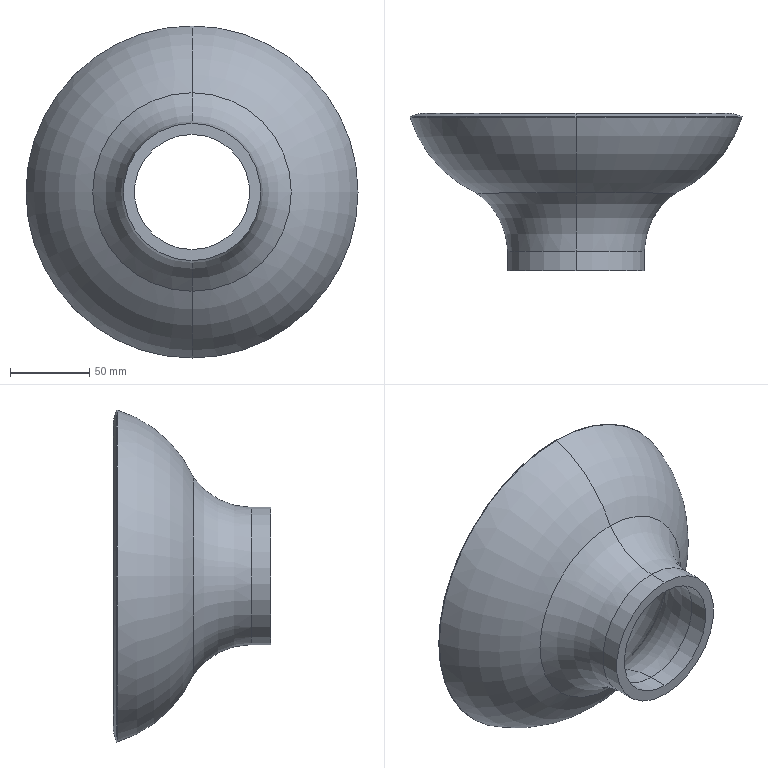Part | SolidWorks | features Revolution 1 | 1 solid | 25 faces | box 209.773 x 99.35 x 209.773 mm | volume 355495 mm3 | torus 14 | cone 6 | cylinder 4 | plane 1 | commonest cylinder face diameters 72.78 x2 86.78 x2
STEP:
#1=CARTESIAN_POINT('',(68.222,-37.326,36.39));
#2=VERTEX_POINT('',#1);
#3=CARTESIAN_POINT('',(68.222,-37.326,-36.39));
#4=VERTEX_POINT('',#3);
#5=CARTESIAN_POINT('',(68.222,-37.326,0.));
#6=DIRECTION('',(0.,-1.,0.));
#7=DIRECTION('',(0.,0.,-1.));
#8=AXIS2_PLACEMENT_3D('',#5,#6,#7);
#9=CIRCLE('',#8,36.39);
#10=EDGE_CURVE('',#2,#4,#9,.T.);
#11=ORIENTED_EDGE('',*,*,#10,.F.);
#12=CARTESIAN_POINT('',(68.222,-49.65,36.39));
#13=VERTEX_POINT('',#12);
#14=CARTESIAN_POINT('',(68.222,-49.65,36.39));
#15=DIRECTION('',(0.,-1.,0.));
#16=VECTOR('',#15,1000.);
#17=LINE('',#14,#16);
#18=EDGE_CURVE('',#2,#13,#17,.T.);
#19=ORIENTED_EDGE('',*,*,#18,.T.);
#20=CARTESIAN_POINT('',(68.222,-49.65,-36.39));
#21=VERTEX_POINT('',#20);
#22=CARTESIAN_POINT('',(68.222,-49.65,0.));
#23=DIRECTION('',(0.,-1.,0.));
#24=DIRECTION('',(0.,0.,-1.));
#25=AXIS2_PLACEMENT_3D('',#22,#23,#24);
#26=CIRCLE('',#25,36.39);
#27=EDGE_CURVE('',#13,#21,#26,.T.);
#28=ORIENTED_EDGE('',*,*,#27,.T.);
#29=CARTESIAN_POINT('',(68.222,-49.65,-36.39));
#30=DIRECTION('',(0.,-1.,0.));
#31=VECTOR('',#30,1000.);
#32=LINE('',#29,#31);
#33=EDGE_CURVE('',#4,#21,#32,.T.);
#34=ORIENTED_EDGE('',*,*,#33,.F.);
#35=EDGE_LOOP('',(#11,#19,#28,#34));
#36=FACE_OUTER_BOUND('',#35,.T.);
#37=CARTESIAN_POINT('',(68.222,-49.65,0.));
#38=DIRECTION('',(0.,-1.,0.));
#39=DIRECTION('',(0.,0.,-1.));
#40=AXIS2_PLACEMENT_3D('',#37,#38,#39);
#41=CYLINDRICAL_SURFACE('',#40,36.39);
#42=ADVANCED_FACE('',(#36),#41,.F.);
#43=CARTESIAN_POINT('',(68.222,-37.326,0.));
#44=DIRECTION('',(0.,-1.,0.));
#45=DIRECTION('',(0.,0.,-1.));
#46=AXIS2_PLACEMENT_3D('',#43,#44,#45);
#47=CIRCLE('',#46,36.39);
#48=EDGE_CURVE('',#4,#2,#47,.T.);
#49=ORIENTED_EDGE('',*,*,#48,.T.);
#50=CARTESIAN_POINT('',(68.222,5.492,59.276));
#51=VERTEX_POINT('',#50);
#52=CARTESIAN_POINT('',(68.222,-37.326,87.887));
#53=DIRECTION('',(1.,0.,0.));
#54=DIRECTION('',(0.,0.,-1.));
#55=AXIS2_PLACEMENT_3D('',#52,#53,#54);
#56=CIRCLE('',#55,51.497);
#57=EDGE_CURVE('',#2,#51,#56,.T.);
#58=ORIENTED_EDGE('',*,*,#57,.T.);
#59=CARTESIAN_POINT('',(68.222,5.492,-59.276));
#60=VERTEX_POINT('',#59);
#61=CARTESIAN_POINT('',(68.222,5.492,0.));
#62=DIRECTION('',(0.,-1.,0.));
#63=DIRECTION('',(0.,0.,-1.));
#64=AXIS2_PLACEMENT_3D('',#61,#62,#63);
#65=CIRCLE('',#64,59.276);
#66=EDGE_CURVE('',#60,#51,#65,.T.);
#67=ORIENTED_EDGE('',*,*,#66,.F.);
#68=CARTESIAN_POINT('',(68.222,-37.326,-87.887));
#69=DIRECTION('',(-1.,0.,0.));
#70=DIRECTION('',(0.,0.,1.));
#71=AXIS2_PLACEMENT_3D('',#68,#69,#70);
#72=CIRCLE('',#71,51.497);
#73=EDGE_CURVE('',#4,#60,#72,.T.);
#74=ORIENTED_EDGE('',*,*,#73,.F.);
#75=EDGE_LOOP('',(#49,#58,#67,#74));
#76=FACE_OUTER_BOUND('',#75,.T.);
#77=CARTESIAN_POINT('',(68.222,-37.326,0.));
#78=DIRECTION('',(0.,-1.,0.));
#79=DIRECTION('',(0.,0.,-1.));
#80=AXIS2_PLACEMENT_3D('',#77,#78,#79);
#81=TOROIDAL_SURFACE('',#80,87.887,51.497);
#82=ADVANCED_FACE('',(#76),#81,.T.);
#83=ORIENTED_EDGE('',*,*,#66,.T.);
#84=CARTESIAN_POINT('',(68.222,5.534,59.352));
#85=VERTEX_POINT('',#84);
#86=CARTESIAN_POINT('',(68.222,5.076,59.553));
#87=DIRECTION('',(1.,0.,0.));
#88=DIRECTION('',(0.,0.,-1.));
#89=AXIS2_PLACEMENT_3D('',#86,#87,#88);
#90=CIRCLE('',#89,0.5);
#91=EDGE_CURVE('',#51,#85,#90,.T.);
#92=ORIENTED_EDGE('',*,*,#91,.T.);
#93=CARTESIAN_POINT('',(68.222,5.534,-59.352));
#94=VERTEX_POINT('',#93);
#95=CARTESIAN_POINT('',(68.222,5.534,0.));
#96=DIRECTION('',(0.,-1.,0.));
#97=DIRECTION('',(0.,0.,-1.));
#98=AXIS2_PLACEMENT_3D('',#95,#96,#97);
#99=CIRCLE('',#98,59.352);
#100=EDGE_CURVE('',#94,#85,#99,.T.);
#101=ORIENTED_EDGE('',*,*,#100,.F.);
#102=CARTESIAN_POINT('',(68.222,5.076,-59.553));
#103=DIRECTION('',(-1.,0.,0.));
#104=DIRECTION('',(0.,0.,1.));
#105=AXIS2_PLACEMENT_3D('',#102,#103,#104);
#106=CIRCLE('',#105,0.5);
#107=EDGE_CURVE('',#60,#94,#106,.T.);
#108=ORIENTED_EDGE('',*,*,#107,.F.);
#109=EDGE_LOOP('',(#83,#92,#101,#108));
#110=FACE_OUTER_BOUND('',#109,.T.);
#111=CARTESIAN_POINT('',(68.222,5.076,0.));
#112=DIRECTION('',(0.,-1.,0.));
#113=DIRECTION('',(0.,0.,-1.));
#114=AXIS2_PLACEMENT_3D('',#111,#112,#113);
#115=TOROIDAL_SURFACE('',#114,59.553,0.5);
#116=ADVANCED_FACE('',(#110),#115,.T.);
#117=CARTESIAN_POINT('',(68.222,49.295,98.116));
#118=VERTEX_POINT('',#117);
#119=CARTESIAN_POINT('',(68.222,49.295,-98.116));
#120=VERTEX_POINT('',#119);
#121=CARTESIAN_POINT('',(68.222,49.295,0.));
#122=DIRECTION('',(0.,-1.,0.));
#123=DIRECTION('',(0.,0.,-1.));
#124=AXIS2_PLACEMENT_3D('',#121,#122,#123);
#125=CIRCLE('',#124,98.116);
#126=EDGE_CURVE('',#118,#120,#125,.T.);
#127=ORIENTED_EDGE('',*,*,#126,.F.);
#128=CARTESIAN_POINT('',(68.222,69.589,31.123));
#129=DIRECTION('',(1.,0.,0.));
#130=DIRECTION('',(0.,0.,-1.));
#131=AXIS2_PLACEMENT_3D('',#128,#129,#130);
#132=CIRCLE('',#131,70.);
#133=EDGE_CURVE('',#118,#85,#132,.T.);
#134=ORIENTED_EDGE('',*,*,#133,.T.);
#135=CARTESIAN_POINT('',(68.222,5.534,0.));
#136=DIRECTION('',(0.,-1.,0.));
#137=DIRECTION('',(0.,0.,-1.));
#138=AXIS2_PLACEMENT_3D('',#135,#136,#137);
#139=CIRCLE('',#138,59.352);
#140=EDGE_CURVE('',#85,#94,#139,.T.);
#141=ORIENTED_EDGE('',*,*,#140,.T.);
#142=CARTESIAN_POINT('',(68.222,69.589,-31.123));
#143=DIRECTION('',(-1.,0.,0.));
#144=DIRECTION('',(0.,0.,1.));
#145=AXIS2_PLACEMENT_3D('',#142,#143,#144);
#146=CIRCLE('',#145,70.);
#147=EDGE_CURVE('',#120,#94,#146,.T.);
#148=ORIENTED_EDGE('',*,*,#147,.F.);
#149=EDGE_LOOP('',(#127,#134,#141,#148));
#150=FACE_OUTER_BOUND('',#149,.T.);
#151=CARTESIAN_POINT('',(68.222,69.589,0.));
#152=DIRECTION('',(0.,-1.,0.));
#153=DIRECTION('',(0.,0.,-1.));
#154=AXIS2_PLACEMENT_3D('',#151,#152,#153);
#155=TOROIDAL_SURFACE('',#154,31.123,70.);
#156=ADVANCED_FACE('',(#150),#155,.F.);
#157=ORIENTED_EDGE('',*,*,#126,.T.);
#158=CARTESIAN_POINT('',(68.222,49.487,-98.174));
#159=VERTEX_POINT('',#158);
#160=CARTESIAN_POINT('',(68.222,49.295,-98.116));
#161=DIRECTION('',(0.,0.9571,-0.2899));
#162=VECTOR('',#161,1000.);
#163=LINE('',#160,#162);
#164=EDGE_CURVE('',#120,#159,#163,.T.);
#165=ORIENTED_EDGE('',*,*,#164,.T.);
#166=CARTESIAN_POINT('',(68.222,49.487,98.174));
#167=VERTEX_POINT('',#166);
#168=CARTESIAN_POINT('',(68.222,49.487,0.));
#169=DIRECTION('',(0.,-1.,0.));
#170=DIRECTION('',(0.,0.,-1.));
#171=AXIS2_PLACEMENT_3D('',#168,#169,#170);
#172=CIRCLE('',#171,98.174);
#173=EDGE_CURVE('',#167,#159,#172,.T.);
#174=ORIENTED_EDGE('',*,*,#173,.F.);
#175=CARTESIAN_POINT('',(68.222,49.295,98.116));
#176=DIRECTION('',(0.,0.9571,0.2899));
#177=VECTOR('',#176,1000.);
#178=LINE('',#175,#177);
#179=EDGE_CURVE('',#118,#167,#178,.T.);
#180=ORIENTED_EDGE('',*,*,#179,.F.);
#181=EDGE_LOOP('',(#157,#165,#174,#180));
#182=FACE_OUTER_BOUND('',#181,.T.);
#183=CARTESIAN_POINT('',(68.222,49.295,0.));
#184=DIRECTION('',(0.,1.,0.));
#185=DIRECTION('',(0.,0.,1.));
#186=AXIS2_PLACEMENT_3D('',#183,#184,#185);
#187=CONICAL_SURFACE('',#186,98.116,0.2941);
#188=ADVANCED_FACE('',(#182),#187,.F.);
#189=CARTESIAN_POINT('',(68.222,49.487,0.));
#190=DIRECTION('',(0.,-1.,0.));
#191=DIRECTION('',(0.,0.,-1.));
#192=AXIS2_PLACEMENT_3D('',#189,#190,#191);
#193=CIRCLE('',#192,98.174);
#194=EDGE_CURVE('',#159,#167,#193,.T.);
#195=ORIENTED_EDGE('',*,*,#194,.T.);
#196=CARTESIAN_POINT('',(68.222,49.687,98.548));
#197=VERTEX_POINT('',#196);
#198=CARTESIAN_POINT('',(68.222,49.4,98.462));
#199=DIRECTION('',(1.,0.,0.));
#200=DIRECTION('',(0.,0.,-1.));
#201=AXIS2_PLACEMENT_3D('',#198,#199,#200);
#202=CIRCLE('',#201,0.3);
#203=EDGE_CURVE('',#167,#197,#202,.T.);
#204=ORIENTED_EDGE('',*,*,#203,.T.);
#205=CARTESIAN_POINT('',(68.222,49.687,-98.548));
#206=VERTEX_POINT('',#205);
#207=CARTESIAN_POINT('',(68.222,49.687,0.));
#208=DIRECTION('',(0.,-1.,0.));
#209=DIRECTION('',(0.,0.,-1.));
#210=AXIS2_PLACEMENT_3D('',#207,#208,#209);
#211=CIRCLE('',#210,98.548);
#212=EDGE_CURVE('',#206,#197,#211,.T.);
#213=ORIENTED_EDGE('',*,*,#212,.F.);
#214=CARTESIAN_POINT('',(68.222,49.4,-98.462));
#215=DIRECTION('',(-1.,0.,0.));
#216=DIRECTION('',(0.,0.,1.));
#217=AXIS2_PLACEMENT_3D('',#214,#215,#216);
#218=CIRCLE('',#217,0.3);
#219=EDGE_CURVE('',#159,#206,#218,.T.);
#220=ORIENTED_EDGE('',*,*,#219,.F.);
#221=EDGE_LOOP('',(#195,#204,#213,#220));
#222=FACE_OUTER_BOUND('',#221,.T.);
#223=CARTESIAN_POINT('',(68.222,49.4,0.));
#224=DIRECTION('',(0.,-1.,0.));
#225=DIRECTION('',(0.,0.,-1.));
#226=AXIS2_PLACEMENT_3D('',#223,#224,#225);
#227=TOROIDAL_SURFACE('',#226,98.462,0.3);
#228=ADVANCED_FACE('',(#222),#227,.T.);
#229=ORIENTED_EDGE('',*,*,#212,.T.);
#230=CARTESIAN_POINT('',(68.222,47.832,104.674));
#231=VERTEX_POINT('',#230);
#232=CARTESIAN_POINT('',(68.222,49.687,98.548));
#233=DIRECTION('',(0.,-0.2899,0.9571));
#234=VECTOR('',#233,1000.);
#235=LINE('',#232,#234);
#236=EDGE_CURVE('',#197,#231,#235,.T.);
#237=ORIENTED_EDGE('',*,*,#236,.T.);
#238=CARTESIAN_POINT('',(68.222,47.832,-104.674));
#239=VERTEX_POINT('',#238);
#240=CARTESIAN_POINT('',(68.222,47.832,0.));
#241=DIRECTION('',(0.,-1.,0.));
#242=DIRECTION('',(0.,0.,-1.));
#243=AXIS2_PLACEMENT_3D('',#240,#241,#242);
#244=CIRCLE('',#243,104.674);
#245=EDGE_CURVE('',#239,#231,#244,.T.);
#246=ORIENTED_EDGE('',*,*,#245,.F.);
#247=CARTESIAN_POINT('',(68.222,49.687,-98.548));
#248=DIRECTION('',(0.,-0.2899,-0.9571));
#249=VECTOR('',#248,1000.);
#250=LINE('',#247,#249);
#251=EDGE_CURVE('',#206,#239,#250,.T.);
#252=ORIENTED_EDGE('',*,*,#251,.F.);
#253=EDGE_LOOP('',(#229,#237,#246,#252));
#254=FACE_OUTER_BOUND('',#253,.T.);
#255=CARTESIAN_POINT('',(68.222,49.687,0.));
#256=DIRECTION('',(0.,-1.,0.));
#257=DIRECTION('',(0.,0.,-1.));
#258=AXIS2_PLACEMENT_3D('',#255,#256,#257);
#259=CONICAL_SURFACE('',#258,98.548,1.277);
#260=ADVANCED_FACE('',(#254),#259,.T.);
#261=ORIENTED_EDGE('',*,*,#245,.T.);
#262=CARTESIAN_POINT('',(68.222,47.457,104.874));
#263=VERTEX_POINT('',#262);
#264=CARTESIAN_POINT('',(68.222,47.544,104.587));
#265=DIRECTION('',(1.,0.,0.));
#266=DIRECTION('',(0.,0.,-1.));
#267=AXIS2_PLACEMENT_3D('',#264,#265,#266);
#268=CIRCLE('',#267,0.3);
#269=EDGE_CURVE('',#231,#263,#268,.T.);
#270=ORIENTED_EDGE('',*,*,#269,.T.);
#271=CARTESIAN_POINT('',(68.222,47.457,-104.874));
#272=VERTEX_POINT('',#271);
#273=CARTESIAN_POINT('',(68.222,47.457,0.));
#274=DIRECTION('',(0.,-1.,0.));
#275=DIRECTION('',(0.,0.,-1.));
#276=AXIS2_PLACEMENT_3D('',#273,#274,#275);
#277=CIRCLE('',#276,104.874);
#278=EDGE_CURVE('',#272,#263,#277,.T.);
#279=ORIENTED_EDGE('',*,*,#278,.F.);
#280=CARTESIAN_POINT('',(68.222,47.544,-104.587));
#281=DIRECTION('',(-1.,0.,0.));
#282=DIRECTION('',(0.,0.,1.));
#283=AXIS2_PLACEMENT_3D('',#280,#281,#282);
#284=CIRCLE('',#283,0.3);
#285=EDGE_CURVE('',#239,#272,#284,.T.);
#286=ORIENTED_EDGE('',*,*,#285,.F.);
#287=EDGE_LOOP('',(#261,#270,#279,#286));
#288=FACE_OUTER_BOUND('',#287,.T.);
#289=CARTESIAN_POINT('',(68.222,47.544,0.));
#290=DIRECTION('',(0.,-1.,0.));
#291=DIRECTION('',(0.,0.,-1.));
#292=AXIS2_PLACEMENT_3D('',#289,#290,#291);
#293=TOROIDAL_SURFACE('',#292,104.587,0.3);
#294=ADVANCED_FACE('',(#288),#293,.T.);
#295=CARTESIAN_POINT('',(68.222,47.266,-104.816));
#296=VERTEX_POINT('',#295);
#297=CARTESIAN_POINT('',(68.222,47.266,104.816));
#298=VERTEX_POINT('',#297);
#299=CARTESIAN_POINT('',(68.222,47.266,0.));
#300=DIRECTION('',(0.,-1.,0.));
#301=DIRECTION('',(0.,0.,-1.));
#302=AXIS2_PLACEMENT_3D('',#299,#300,#301);
#303=CIRCLE('',#302,104.816);
#304=EDGE_CURVE('',#296,#298,#303,.T.);
#305=ORIENTED_EDGE('',*,*,#304,.F.);
#306=CARTESIAN_POINT('',(68.222,47.457,-104.874));
#307=DIRECTION('',(0.,0.9571,-0.2899));
#308=VECTOR('',#307,1000.);
#309=LINE('',#306,#308);
#310=EDGE_CURVE('',#296,#272,#309,.T.);
#311=ORIENTED_EDGE('',*,*,#310,.T.);
#312=ORIENTED_EDGE('',*,*,#278,.T.);
#313=CARTESIAN_POINT('',(68.222,47.457,104.874));
#314=DIRECTION('',(0.,0.9571,0.2899));
#315=VECTOR('',#314,1000.);
#316=LINE('',#313,#315);
#317=EDGE_CURVE('',#298,#263,#316,.T.);
#318=ORIENTED_EDGE('',*,*,#317,.F.);
#319=EDGE_LOOP('',(#305,#311,#312,#318));
#320=FACE_OUTER_BOUND('',#319,.T.);
#321=CARTESIAN_POINT('',(68.222,47.457,0.));
#322=DIRECTION('',(0.,1.,0.));
#323=DIRECTION('',(0.,0.,1.));
#324=AXIS2_PLACEMENT_3D('',#321,#322,#323);
#325=CONICAL_SURFACE('',#324,104.874,0.2941);
#326=ADVANCED_FACE('',(#320),#325,.T.);
#327=ORIENTED_EDGE('',*,*,#304,.T.);
#328=CARTESIAN_POINT('',(68.222,-0.6284,62.722));
#329=VERTEX_POINT('',#328);
#330=CARTESIAN_POINT('',(68.222,69.589,31.123));
#331=DIRECTION('',(1.,0.,0.));
#332=DIRECTION('',(0.,0.,-1.));
#333=AXIS2_PLACEMENT_3D('',#330,#331,#332);
#334=CIRCLE('',#333,77.);
#335=EDGE_CURVE('',#298,#329,#334,.T.);
#336=ORIENTED_EDGE('',*,*,#335,.T.);
#337=CARTESIAN_POINT('',(68.222,-0.6284,-62.722));
#338=VERTEX_POINT('',#337);
#339=CARTESIAN_POINT('',(68.222,-0.6284,0.));
#340=DIRECTION('',(0.,-1.,0.));
#341=DIRECTION('',(0.,0.,-1.));
#342=AXIS2_PLACEMENT_3D('',#339,#340,#341);
#343=CIRCLE('',#342,62.722);
#344=EDGE_CURVE('',#338,#329,#343,.T.);
#345=ORIENTED_EDGE('',*,*,#344,.F.);
#346=CARTESIAN_POINT('',(68.222,69.589,-31.123));
#347=DIRECTION('',(-1.,0.,0.));
#348=DIRECTION('',(0.,0.,1.));
#349=AXIS2_PLACEMENT_3D('',#346,#347,#348);
#350=CIRCLE('',#349,77.);
#351=EDGE_CURVE('',#296,#338,#350,.T.);
#352=ORIENTED_EDGE('',*,*,#351,.F.);
#353=EDGE_LOOP('',(#327,#336,#345,#352));
#354=FACE_OUTER_BOUND('',#353,.T.);
#355=CARTESIAN_POINT('',(68.222,69.589,0.));
#356=DIRECTION('',(0.,-1.,0.));
#357=DIRECTION('',(0.,0.,-1.));
#358=AXIS2_PLACEMENT_3D('',#355,#356,#357);
#359=TOROIDAL_SURFACE('',#358,31.123,77.);
#360=ADVANCED_FACE('',(#354),#359,.T.);
#361=CARTESIAN_POINT('',(68.222,-37.326,43.39));
#362=VERTEX_POINT('',#361);
#363=CARTESIAN_POINT('',(68.222,-37.326,-43.39));
#364=VERTEX_POINT('',#363);
#365=CARTESIAN_POINT('',(68.222,-37.326,0.));
#366=DIRECTION('',(0.,-1.,0.));
#367=DIRECTION('',(0.,0.,-1.));
#368=AXIS2_PLACEMENT_3D('',#365,#366,#367);
#369=CIRCLE('',#368,43.39);
#370=EDGE_CURVE('',#362,#364,#369,.T.);
#371=ORIENTED_EDGE('',*,*,#370,.F.);
#372=CARTESIAN_POINT('',(68.222,-37.326,87.887));
#373=DIRECTION('',(1.,0.,0.));
#374=DIRECTION('',(0.,0.,-1.));
#375=AXIS2_PLACEMENT_3D('',#372,#373,#374);
#376=CIRCLE('',#375,44.497);
#377=EDGE_CURVE('',#362,#329,#376,.T.);
#378=ORIENTED_EDGE('',*,*,#377,.T.);
#379=CARTESIAN_POINT('',(68.222,-0.6284,0.));
#380=DIRECTION('',(0.,-1.,0.));
#381=DIRECTION('',(0.,0.,-1.));
#382=AXIS2_PLACEMENT_3D('',#379,#380,#381);
#383=CIRCLE('',#382,62.722);
#384=EDGE_CURVE('',#329,#338,#383,.T.);
#385=ORIENTED_EDGE('',*,*,#384,.T.);
#386=CARTESIAN_POINT('',(68.222,-37.326,-87.887));
#387=DIRECTION('',(-1.,0.,0.));
#388=DIRECTION('',(0.,0.,1.));
#389=AXIS2_PLACEMENT_3D('',#386,#387,#388);
#390=CIRCLE('',#389,44.497);
#391=EDGE_CURVE('',#364,#338,#390,.T.);
#392=ORIENTED_EDGE('',*,*,#391,.F.);
#393=EDGE_LOOP('',(#371,#378,#385,#392));
#394=FACE_OUTER_BOUND('',#393,.T.);
#395=CARTESIAN_POINT('',(68.222,-37.326,0.));
#396=DIRECTION('',(0.,-1.,0.));
#397=DIRECTION('',(0.,0.,-1.));
#398=AXIS2_PLACEMENT_3D('',#395,#396,#397);
#399=TOROIDAL_SURFACE('',#398,87.887,44.497);
#400=ADVANCED_FACE('',(#394),#399,.F.);
#401=CARTESIAN_POINT('',(68.222,-37.326,0.));
#402=DIRECTION('',(0.,-1.,0.));
#403=DIRECTION('',(0.,0.,-1.));
#404=AXIS2_PLACEMENT_3D('',#401,#402,#403);
#405=CIRCLE('',#404,43.39);
#406=EDGE_CURVE('',#364,#362,#405,.T.);
#407=ORIENTED_EDGE('',*,*,#406,.T.);
#408=CARTESIAN_POINT('',(68.222,-49.65,43.39));
#409=VERTEX_POINT('',#408);
#410=CARTESIAN_POINT('',(68.222,-49.65,43.39));
#411=DIRECTION('',(0.,-1.,0.));
#412=VECTOR('',#411,1000.);
#413=LINE('',#410,#412);
#414=EDGE_CURVE('',#362,#409,#413,.T.);
#415=ORIENTED_EDGE('',*,*,#414,.T.);
#416=CARTESIAN_POINT('',(68.222,-49.65,-43.39));
#417=VERTEX_POINT('',#416);
#418=CARTESIAN_POINT('',(68.222,-49.65,0.));
#419=DIRECTION('',(0.,-1.,0.));
#420=DIRECTION('',(0.,0.,-1.));
#421=AXIS2_PLACEMENT_3D('',#418,#419,#420);
#422=CIRCLE('',#421,43.39);
#423=EDGE_CURVE('',#417,#409,#422,.T.);
#424=ORIENTED_EDGE('',*,*,#423,.F.);
#425=CARTESIAN_POINT('',(68.222,-49.65,-43.39));
#426=DIRECTION('',(0.,-1.,0.));
#427=VECTOR('',#426,1000.);
#428=LINE('',#425,#427);
#429=EDGE_CURVE('',#364,#417,#428,.T.);
#430=ORIENTED_EDGE('',*,*,#429,.F.);
#431=EDGE_LOOP('',(#407,#415,#424,#430));
#432=FACE_OUTER_BOUND('',#431,.T.);
#433=CARTESIAN_POINT('',(68.222,-49.65,0.));
#434=DIRECTION('',(0.,-1.,0.));
#435=DIRECTION('',(0.,0.,-1.));
#436=AXIS2_PLACEMENT_3D('',#433,#434,#435);
#437=CYLINDRICAL_SURFACE('',#436,43.39);
#438=ADVANCED_FACE('',(#432),#437,.T.);
#439=CARTESIAN_POINT('',(68.222,-49.65,0.));
#440=DIRECTION('',(0.,-1.,0.));
#441=DIRECTION('',(0.,0.,-1.));
#442=AXIS2_PLACEMENT_3D('',#439,#440,#441);
#443=CIRCLE('',#442,36.39);
#444=EDGE_CURVE('',#21,#13,#443,.T.);
#445=ORIENTED_EDGE('',*,*,#444,.F.);
#446=ORIENTED_EDGE('',*,*,#27,.F.);
#447=EDGE_LOOP('',(#445,#446));
#448=FACE_BOUND('',#447,.T.);
#449=ORIENTED_EDGE('',*,*,#423,.T.);
#450=CARTESIAN_POINT('',(68.222,-49.65,0.));
#451=DIRECTION('',(0.,-1.,0.));
#452=DIRECTION('',(0.,0.,-1.));
#453=AXIS2_PLACEMENT_3D('',#450,#451,#452);
#454=CIRCLE('',#453,43.39);
#455=EDGE_CURVE('',#409,#417,#454,.T.);
#456=ORIENTED_EDGE('',*,*,#455,.T.);
#457=EDGE_LOOP('',(#449,#456));
#458=FACE_OUTER_BOUND('',#457,.T.);
#459=CARTESIAN_POINT('',(24.832,-49.65,0.));
#460=DIRECTION('',(0.,1.,0.));
#461=DIRECTION('',(0.,0.,1.));
#462=AXIS2_PLACEMENT_3D('',#459,#460,#461);
#463=PLANE('',#462);
#464=ADVANCED_FACE('',(#448,#458),#463,.F.);
#465=ORIENTED_EDGE('',*,*,#414,.F.);
#466=ORIENTED_EDGE('',*,*,#370,.T.);
#467=ORIENTED_EDGE('',*,*,#429,.T.);
#468=ORIENTED_EDGE('',*,*,#455,.F.);
#469=EDGE_LOOP('',(#465,#466,#467,#468));
#470=FACE_OUTER_BOUND('',#469,.T.);
#471=CARTESIAN_POINT('',(68.222,-49.65,0.));
#472=DIRECTION('',(0.,-1.,0.));
#473=DIRECTION('',(0.,0.,-1.));
#474=AXIS2_PLACEMENT_3D('',#471,#472,#473);
#475=CYLINDRICAL_SURFACE('',#474,43.39);
#476=ADVANCED_FACE('',(#470),#475,.T.);
#477=ORIENTED_EDGE('',*,*,#377,.F.);
#478=ORIENTED_EDGE('',*,*,#406,.F.);
#479=ORIENTED_EDGE('',*,*,#391,.T.);
#480=ORIENTED_EDGE('',*,*,#344,.T.);
#481=EDGE_LOOP('',(#477,#478,#479,#480));
#482=FACE_OUTER_BOUND('',#481,.T.);
#483=CARTESIAN_POINT('',(68.222,-37.326,0.));
#484=DIRECTION('',(0.,-1.,0.));
#485=DIRECTION('',(0.,0.,-1.));
#486=AXIS2_PLACEMENT_3D('',#483,#484,#485);
#487=TOROIDAL_SURFACE('',#486,87.887,44.497);
#488=ADVANCED_FACE('',(#482),#487,.F.);
#489=ORIENTED_EDGE('',*,*,#335,.F.);
#490=CARTESIAN_POINT('',(68.222,47.266,0.));
#491=DIRECTION('',(0.,-1.,0.));
#492=DIRECTION('',(0.,0.,-1.));
#493=AXIS2_PLACEMENT_3D('',#490,#491,#492);
#494=CIRCLE('',#493,104.816);
#495=EDGE_CURVE('',#298,#296,#494,.T.);
#496=ORIENTED_EDGE('',*,*,#495,.T.);
#497=ORIENTED_EDGE('',*,*,#351,.T.);
#498=ORIENTED_EDGE('',*,*,#384,.F.);
#499=EDGE_LOOP('',(#489,#496,#497,#498));
#500=FACE_OUTER_BOUND('',#499,.T.);
#501=CARTESIAN_POINT('',(68.222,69.589,0.));
#502=DIRECTION('',(0.,-1.,0.));
#503=DIRECTION('',(0.,0.,-1.));
#504=AXIS2_PLACEMENT_3D('',#501,#502,#503);
#505=TOROIDAL_SURFACE('',#504,31.123,77.);
#506=ADVANCED_FACE('',(#500),#505,.T.);
#507=ORIENTED_EDGE('',*,*,#310,.F.);
#508=ORIENTED_EDGE('',*,*,#495,.F.);
#509=ORIENTED_EDGE('',*,*,#317,.T.);
#510=CARTESIAN_POINT('',(68.222,47.457,0.));
#511=DIRECTION('',(0.,-1.,0.));
#512=DIRECTION('',(0.,0.,-1.));
#513=AXIS2_PLACEMENT_3D('',#510,#511,#512);
#514=CIRCLE('',#513,104.874);
#515=EDGE_CURVE('',#263,#272,#514,.T.);
#516=ORIENTED_EDGE('',*,*,#515,.T.);
#517=EDGE_LOOP('',(#507,#508,#509,#516));
#518=FACE_OUTER_BOUND('',#517,.T.);
#519=CARTESIAN_POINT('',(68.222,47.457,0.));
#520=DIRECTION('',(0.,1.,0.));
#521=DIRECTION('',(0.,0.,1.));
#522=AXIS2_PLACEMENT_3D('',#519,#520,#521);
#523=CONICAL_SURFACE('',#522,104.874,0.2941);
#524=ADVANCED_FACE('',(#518),#523,.T.);
#525=ORIENTED_EDGE('',*,*,#269,.F.);
#526=CARTESIAN_POINT('',(68.222,47.832,0.));
#527=DIRECTION('',(0.,-1.,0.));
#528=DIRECTION('',(0.,0.,-1.));
#529=AXIS2_PLACEMENT_3D('',#526,#527,#528);
#530=CIRCLE('',#529,104.674);
#531=EDGE_CURVE('',#231,#239,#530,.T.);
#532=ORIENTED_EDGE('',*,*,#531,.T.);
#533=ORIENTED_EDGE('',*,*,#285,.T.);
#534=ORIENTED_EDGE('',*,*,#515,.F.);
#535=EDGE_LOOP('',(#525,#532,#533,#534));
#536=FACE_OUTER_BOUND('',#535,.T.);
#537=CARTESIAN_POINT('',(68.222,47.544,0.));
#538=DIRECTION('',(0.,-1.,0.));
#539=DIRECTION('',(0.,0.,-1.));
#540=AXIS2_PLACEMENT_3D('',#537,#538,#539);
#541=TOROIDAL_SURFACE('',#540,104.587,0.3);
#542=ADVANCED_FACE('',(#536),#541,.T.);
#543=ORIENTED_EDGE('',*,*,#236,.F.);
#544=CARTESIAN_POINT('',(68.222,49.687,0.));
#545=DIRECTION('',(0.,-1.,0.));
#546=DIRECTION('',(0.,0.,-1.));
#547=AXIS2_PLACEMENT_3D('',#544,#545,#546);
#548=CIRCLE('',#547,98.548);
#549=EDGE_CURVE('',#197,#206,#548,.T.);
#550=ORIENTED_EDGE('',*,*,#549,.T.);
#551=ORIENTED_EDGE('',*,*,#251,.T.);
#552=ORIENTED_EDGE('',*,*,#531,.F.);
#553=EDGE_LOOP('',(#543,#550,#551,#552));
#554=FACE_OUTER_BOUND('',#553,.T.);
#555=CARTESIAN_POINT('',(68.222,49.687,0.));
#556=DIRECTION('',(0.,-1.,0.));
#557=DIRECTION('',(0.,0.,-1.));
#558=AXIS2_PLACEMENT_3D('',#555,#556,#557);
#559=CONICAL_SURFACE('',#558,98.548,1.277);
#560=ADVANCED_FACE('',(#554),#559,.T.);
#561=ORIENTED_EDGE('',*,*,#203,.F.);
#562=ORIENTED_EDGE('',*,*,#173,.T.);
#563=ORIENTED_EDGE('',*,*,#219,.T.);
#564=ORIENTED_EDGE('',*,*,#549,.F.);
#565=EDGE_LOOP('',(#561,#562,#563,#564));
#566=FACE_OUTER_BOUND('',#565,.T.);
#567=CARTESIAN_POINT('',(68.222,49.4,0.));
#568=DIRECTION('',(0.,-1.,0.));
#569=DIRECTION('',(0.,0.,-1.));
#570=AXIS2_PLACEMENT_3D('',#567,#568,#569);
#571=TOROIDAL_SURFACE('',#570,98.462,0.3);
#572=ADVANCED_FACE('',(#566),#571,.T.);
#573=ORIENTED_EDGE('',*,*,#164,.F.);
#574=CARTESIAN_POINT('',(68.222,49.295,0.));
#575=DIRECTION('',(0.,-1.,0.));
#576=DIRECTION('',(0.,0.,-1.));
#577=AXIS2_PLACEMENT_3D('',#574,#575,#576);
#578=CIRCLE('',#577,98.116);
#579=EDGE_CURVE('',#120,#118,#578,.T.);
#580=ORIENTED_EDGE('',*,*,#579,.T.);
#581=ORIENTED_EDGE('',*,*,#179,.T.);
#582=ORIENTED_EDGE('',*,*,#194,.F.);
#583=EDGE_LOOP('',(#573,#580,#581,#582));
#584=FACE_OUTER_BOUND('',#583,.T.);
#585=CARTESIAN_POINT('',(68.222,49.295,0.));
#586=DIRECTION('',(0.,1.,0.));
#587=DIRECTION('',(0.,0.,1.));
#588=AXIS2_PLACEMENT_3D('',#585,#586,#587);
#589=CONICAL_SURFACE('',#588,98.116,0.2941);
#590=ADVANCED_FACE('',(#584),#589,.F.);
#591=ORIENTED_EDGE('',*,*,#133,.F.);
#592=ORIENTED_EDGE('',*,*,#579,.F.);
#593=ORIENTED_EDGE('',*,*,#147,.T.);
#594=ORIENTED_EDGE('',*,*,#100,.T.);
#595=EDGE_LOOP('',(#591,#592,#593,#594));
#596=FACE_OUTER_BOUND('',#595,.T.);
#597=CARTESIAN_POINT('',(68.222,69.589,0.));
#598=DIRECTION('',(0.,-1.,0.));
#599=DIRECTION('',(0.,0.,-1.));
#600=AXIS2_PLACEMENT_3D('',#597,#598,#599);
#601=TOROIDAL_SURFACE('',#600,31.123,70.);
#602=ADVANCED_FACE('',(#596),#601,.F.);
#603=ORIENTED_EDGE('',*,*,#91,.F.);
#604=CARTESIAN_POINT('',(68.222,5.492,0.));
#605=DIRECTION('',(0.,-1.,0.));
#606=DIRECTION('',(0.,0.,-1.));
#607=AXIS2_PLACEMENT_3D('',#604,#605,#606);
#608=CIRCLE('',#607,59.276);
#609=EDGE_CURVE('',#51,#60,#608,.T.);
#610=ORIENTED_EDGE('',*,*,#609,.T.);
#611=ORIENTED_EDGE('',*,*,#107,.T.);
#612=ORIENTED_EDGE('',*,*,#140,.F.);
#613=EDGE_LOOP('',(#603,#610,#611,#612));
#614=FACE_OUTER_BOUND('',#613,.T.);
#615=CARTESIAN_POINT('',(68.222,5.076,0.));
#616=DIRECTION('',(0.,-1.,0.));
#617=DIRECTION('',(0.,0.,-1.));
#618=AXIS2_PLACEMENT_3D('',#615,#616,#617);
#619=TOROIDAL_SURFACE('',#618,59.553,0.5);
#620=ADVANCED_FACE('',(#614),#619,.T.);
#621=ORIENTED_EDGE('',*,*,#57,.F.);
#622=ORIENTED_EDGE('',*,*,#10,.T.);
#623=ORIENTED_EDGE('',*,*,#73,.T.);
#624=ORIENTED_EDGE('',*,*,#609,.F.);
#625=EDGE_LOOP('',(#621,#622,#623,#624));
#626=FACE_OUTER_BOUND('',#625,.T.);
#627=CARTESIAN_POINT('',(68.222,-37.326,0.));
#628=DIRECTION('',(0.,-1.,0.));
#629=DIRECTION('',(0.,0.,-1.));
#630=AXIS2_PLACEMENT_3D('',#627,#628,#629);
#631=TOROIDAL_SURFACE('',#630,87.887,51.497);
#632=ADVANCED_FACE('',(#626),#631,.T.);
#633=ORIENTED_EDGE('',*,*,#18,.F.);
#634=ORIENTED_EDGE('',*,*,#48,.F.);
#635=ORIENTED_EDGE('',*,*,#33,.T.);
#636=ORIENTED_EDGE('',*,*,#444,.T.);
#637=EDGE_LOOP('',(#633,#634,#635,#636));
#638=FACE_OUTER_BOUND('',#637,.T.);
#639=CARTESIAN_POINT('',(68.222,-49.65,0.));
#640=DIRECTION('',(0.,-1.,0.));
#641=DIRECTION('',(0.,0.,-1.));
#642=AXIS2_PLACEMENT_3D('',#639,#640,#641);
#643=CYLINDRICAL_SURFACE('',#642,36.39);
#644=ADVANCED_FACE('',(#638),#643,.F.);
#645=CLOSED_SHELL('',(#42,#82,#116,#156,#188,#228,#260,#294,#326,#360,#400,#438,#464,#476,#488,#506,#524,#542,#560,#572,#590,#602,#620,#632,#644));
#646=MANIFOLD_SOLID_BREP('',#645);
#647=CARTESIAN_POINT('',(0.,0.,0.));
#648=DIRECTION('',(0.,0.,1.));
#649=DIRECTION('',(1.,0.,0.));
#650=AXIS2_PLACEMENT_3D('',#647,#648,#649);
#651=(LENGTH_UNIT()NAMED_UNIT(*)SI_UNIT(.MILLI.,.METRE.));
#652=UNCERTAINTY_MEASURE_WITH_UNIT(LENGTH_MEASURE(0.00001),#651,'','');
#653=(NAMED_UNIT(*)PLANE_ANGLE_UNIT()SI_UNIT($,.RADIAN.));
#654=(NAMED_UNIT(*)SI_UNIT($,.STERADIAN.)SOLID_ANGLE_UNIT());
#655=(GEOMETRIC_REPRESENTATION_CONTEXT(3)GLOBAL_UNCERTAINTY_ASSIGNED_CONTEXT((#652))GLOBAL_UNIT_ASSIGNED_CONTEXT((#651,#653,#654))REPRESENTATION_CONTEXT('',''));
#656=ADVANCED_BREP_SHAPE_REPRESENTATION('',(#646,#650),#655);